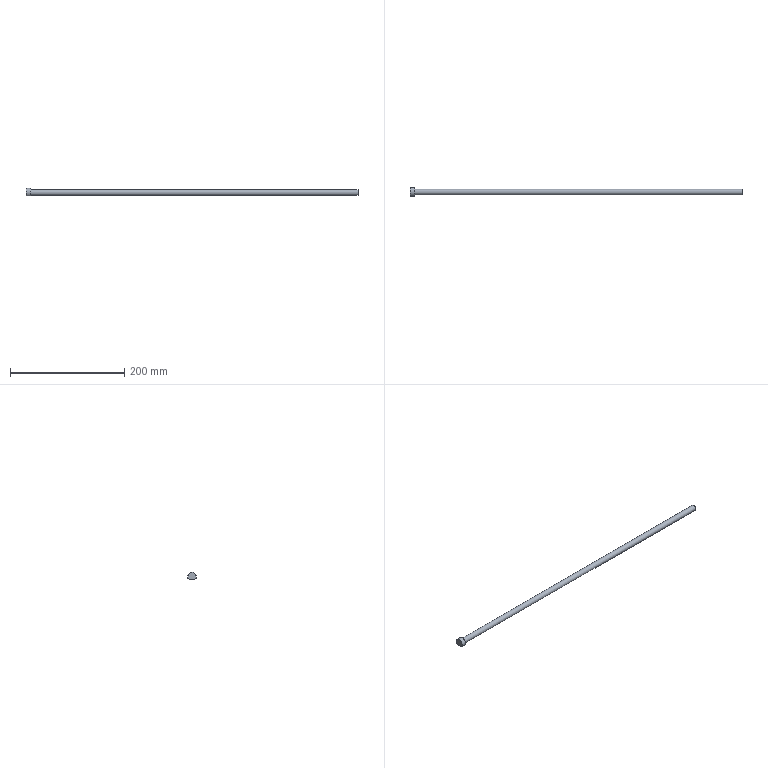Part | STEP file | solid 35 | 1 solid | 6 faces | box 580 x 15 x 13 mm | volume 46226 mm3 | plane 4 | cylinder 2 | commonest cylinder face diameters 10 x1 15 x1